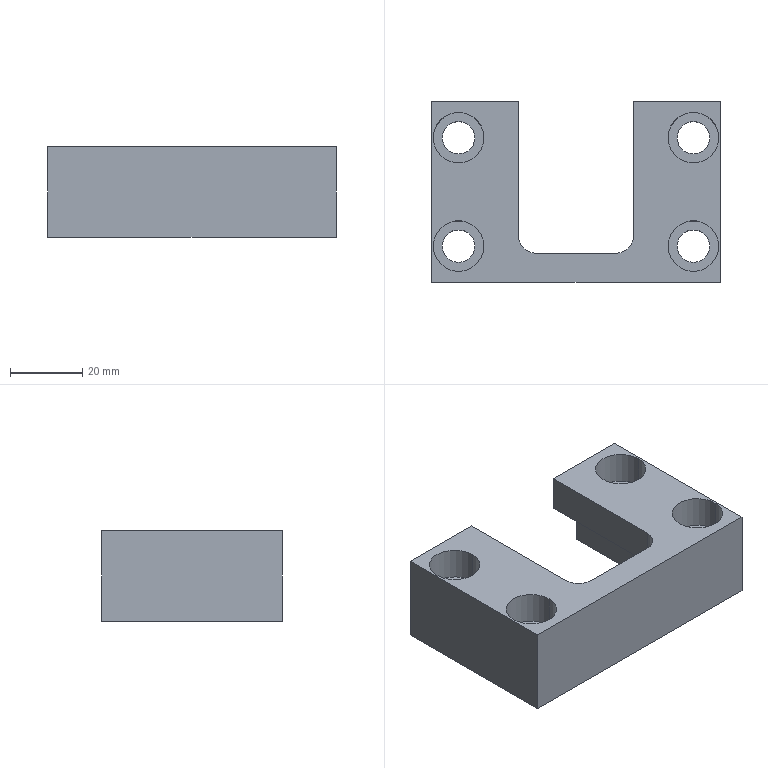Part | SolidWorks | features BaseBody 1 | 1 solid | 38 faces | box 80 x 50 x 25 mm | volume 45715 mm3 | cylinder 20 | plane 18 | commonest cylinder face diameters 9 x8 14 x8 10 x4
STEP:
#1=CARTESIAN_POINT('',(25.5,15.,3.5));
#2=VERTEX_POINT('',#1);
#3=CARTESIAN_POINT('',(39.5,15.,3.5));
#4=VERTEX_POINT('',#3);
#5=CARTESIAN_POINT('',(32.5,15.,3.5));
#6=DIRECTION('',(0.,0.,1.));
#7=DIRECTION('',(1.,0.,0.));
#8=AXIS2_PLACEMENT_3D('',#5,#6,#7);
#9=CIRCLE('',#8,7.);
#10=EDGE_CURVE('',#2,#4,#9,.T.);
#11=ORIENTED_EDGE('',*,*,#10,.F.);
#12=CARTESIAN_POINT('',(25.5,15.,12.5));
#13=VERTEX_POINT('',#12);
#14=CARTESIAN_POINT('',(25.5,15.,12.5));
#15=DIRECTION('',(0.,0.,1.));
#16=VECTOR('',#15,1000.);
#17=LINE('',#14,#16);
#18=EDGE_CURVE('',#2,#13,#17,.T.);
#19=ORIENTED_EDGE('',*,*,#18,.T.);
#20=CARTESIAN_POINT('',(39.5,15.,12.5));
#21=VERTEX_POINT('',#20);
#22=CARTESIAN_POINT('',(32.5,15.,12.5));
#23=DIRECTION('',(0.,0.,1.));
#24=DIRECTION('',(1.,0.,0.));
#25=AXIS2_PLACEMENT_3D('',#22,#23,#24);
#26=CIRCLE('',#25,7.);
#27=EDGE_CURVE('',#13,#21,#26,.T.);
#28=ORIENTED_EDGE('',*,*,#27,.T.);
#29=CARTESIAN_POINT('',(39.5,15.,12.5));
#30=DIRECTION('',(0.,0.,1.));
#31=VECTOR('',#30,1000.);
#32=LINE('',#29,#31);
#33=EDGE_CURVE('',#4,#21,#32,.T.);
#34=ORIENTED_EDGE('',*,*,#33,.F.);
#35=EDGE_LOOP('',(#11,#19,#28,#34));
#36=FACE_OUTER_BOUND('',#35,.T.);
#37=CARTESIAN_POINT('',(32.5,15.,12.5));
#38=DIRECTION('',(0.,0.,1.));
#39=DIRECTION('',(1.,0.,0.));
#40=AXIS2_PLACEMENT_3D('',#37,#38,#39);
#41=CYLINDRICAL_SURFACE('',#40,7.);
#42=ADVANCED_FACE('',(#36),#41,.F.);
#43=CARTESIAN_POINT('',(28.,15.,-12.5));
#44=VERTEX_POINT('',#43);
#45=CARTESIAN_POINT('',(37.,15.,-12.5));
#46=VERTEX_POINT('',#45);
#47=CARTESIAN_POINT('',(32.5,15.,-12.5));
#48=DIRECTION('',(0.,0.,1.));
#49=DIRECTION('',(1.,0.,0.));
#50=AXIS2_PLACEMENT_3D('',#47,#48,#49);
#51=CIRCLE('',#50,4.5);
#52=EDGE_CURVE('',#44,#46,#51,.T.);
#53=ORIENTED_EDGE('',*,*,#52,.F.);
#54=CARTESIAN_POINT('',(28.,15.,3.5));
#55=VERTEX_POINT('',#54);
#56=CARTESIAN_POINT('',(28.,15.,12.5));
#57=DIRECTION('',(0.,0.,1.));
#58=VECTOR('',#57,1000.);
#59=LINE('',#56,#58);
#60=EDGE_CURVE('',#44,#55,#59,.T.);
#61=ORIENTED_EDGE('',*,*,#60,.T.);
#62=CARTESIAN_POINT('',(37.,15.,3.5));
#63=VERTEX_POINT('',#62);
#64=CARTESIAN_POINT('',(32.5,15.,3.5));
#65=DIRECTION('',(0.,0.,1.));
#66=DIRECTION('',(1.,0.,0.));
#67=AXIS2_PLACEMENT_3D('',#64,#65,#66);
#68=CIRCLE('',#67,4.5);
#69=EDGE_CURVE('',#55,#63,#68,.T.);
#70=ORIENTED_EDGE('',*,*,#69,.T.);
#71=CARTESIAN_POINT('',(37.,15.,12.5));
#72=DIRECTION('',(0.,0.,1.));
#73=VECTOR('',#72,1000.);
#74=LINE('',#71,#73);
#75=EDGE_CURVE('',#46,#63,#74,.T.);
#76=ORIENTED_EDGE('',*,*,#75,.F.);
#77=EDGE_LOOP('',(#53,#61,#70,#76));
#78=FACE_OUTER_BOUND('',#77,.T.);
#79=CARTESIAN_POINT('',(32.5,15.,12.5));
#80=DIRECTION('',(0.,0.,1.));
#81=DIRECTION('',(1.,0.,0.));
#82=AXIS2_PLACEMENT_3D('',#79,#80,#81);
#83=CYLINDRICAL_SURFACE('',#82,4.5);
#84=ADVANCED_FACE('',(#78),#83,.F.);
#85=CARTESIAN_POINT('',(25.5,-15.,3.5));
#86=VERTEX_POINT('',#85);
#87=CARTESIAN_POINT('',(39.5,-15.,3.5));
#88=VERTEX_POINT('',#87);
#89=CARTESIAN_POINT('',(32.5,-15.,3.5));
#90=DIRECTION('',(0.,0.,1.));
#91=DIRECTION('',(1.,0.,0.));
#92=AXIS2_PLACEMENT_3D('',#89,#90,#91);
#93=CIRCLE('',#92,7.);
#94=EDGE_CURVE('',#86,#88,#93,.T.);
#95=ORIENTED_EDGE('',*,*,#94,.F.);
#96=CARTESIAN_POINT('',(25.5,-15.,12.5));
#97=VERTEX_POINT('',#96);
#98=CARTESIAN_POINT('',(25.5,-15.,12.5));
#99=DIRECTION('',(0.,0.,1.));
#100=VECTOR('',#99,1000.);
#101=LINE('',#98,#100);
#102=EDGE_CURVE('',#86,#97,#101,.T.);
#103=ORIENTED_EDGE('',*,*,#102,.T.);
#104=CARTESIAN_POINT('',(39.5,-15.,12.5));
#105=VERTEX_POINT('',#104);
#106=CARTESIAN_POINT('',(32.5,-15.,12.5));
#107=DIRECTION('',(0.,0.,1.));
#108=DIRECTION('',(1.,0.,0.));
#109=AXIS2_PLACEMENT_3D('',#106,#107,#108);
#110=CIRCLE('',#109,7.);
#111=EDGE_CURVE('',#97,#105,#110,.T.);
#112=ORIENTED_EDGE('',*,*,#111,.T.);
#113=CARTESIAN_POINT('',(39.5,-15.,12.5));
#114=DIRECTION('',(0.,0.,1.));
#115=VECTOR('',#114,1000.);
#116=LINE('',#113,#115);
#117=EDGE_CURVE('',#88,#105,#116,.T.);
#118=ORIENTED_EDGE('',*,*,#117,.F.);
#119=EDGE_LOOP('',(#95,#103,#112,#118));
#120=FACE_OUTER_BOUND('',#119,.T.);
#121=CARTESIAN_POINT('',(32.5,-15.,12.5));
#122=DIRECTION('',(0.,0.,1.));
#123=DIRECTION('',(1.,0.,0.));
#124=AXIS2_PLACEMENT_3D('',#121,#122,#123);
#125=CYLINDRICAL_SURFACE('',#124,7.);
#126=ADVANCED_FACE('',(#120),#125,.F.);
#127=CARTESIAN_POINT('',(28.,-15.,-12.5));
#128=VERTEX_POINT('',#127);
#129=CARTESIAN_POINT('',(37.,-15.,-12.5));
#130=VERTEX_POINT('',#129);
#131=CARTESIAN_POINT('',(32.5,-15.,-12.5));
#132=DIRECTION('',(0.,0.,1.));
#133=DIRECTION('',(1.,0.,0.));
#134=AXIS2_PLACEMENT_3D('',#131,#132,#133);
#135=CIRCLE('',#134,4.5);
#136=EDGE_CURVE('',#128,#130,#135,.T.);
#137=ORIENTED_EDGE('',*,*,#136,.F.);
#138=CARTESIAN_POINT('',(28.,-15.,3.5));
#139=VERTEX_POINT('',#138);
#140=CARTESIAN_POINT('',(28.,-15.,12.5));
#141=DIRECTION('',(0.,0.,1.));
#142=VECTOR('',#141,1000.);
#143=LINE('',#140,#142);
#144=EDGE_CURVE('',#128,#139,#143,.T.);
#145=ORIENTED_EDGE('',*,*,#144,.T.);
#146=CARTESIAN_POINT('',(37.,-15.,3.5));
#147=VERTEX_POINT('',#146);
#148=CARTESIAN_POINT('',(32.5,-15.,3.5));
#149=DIRECTION('',(0.,0.,1.));
#150=DIRECTION('',(1.,0.,0.));
#151=AXIS2_PLACEMENT_3D('',#148,#149,#150);
#152=CIRCLE('',#151,4.5);
#153=EDGE_CURVE('',#139,#147,#152,.T.);
#154=ORIENTED_EDGE('',*,*,#153,.T.);
#155=CARTESIAN_POINT('',(37.,-15.,12.5));
#156=DIRECTION('',(0.,0.,1.));
#157=VECTOR('',#156,1000.);
#158=LINE('',#155,#157);
#159=EDGE_CURVE('',#130,#147,#158,.T.);
#160=ORIENTED_EDGE('',*,*,#159,.F.);
#161=EDGE_LOOP('',(#137,#145,#154,#160));
#162=FACE_OUTER_BOUND('',#161,.T.);
#163=CARTESIAN_POINT('',(32.5,-15.,12.5));
#164=DIRECTION('',(0.,0.,1.));
#165=DIRECTION('',(1.,0.,0.));
#166=AXIS2_PLACEMENT_3D('',#163,#164,#165);
#167=CYLINDRICAL_SURFACE('',#166,4.5);
#168=ADVANCED_FACE('',(#162),#167,.F.);
#169=CARTESIAN_POINT('',(-39.5,15.,3.5));
#170=VERTEX_POINT('',#169);
#171=CARTESIAN_POINT('',(-25.5,15.,3.5));
#172=VERTEX_POINT('',#171);
#173=CARTESIAN_POINT('',(-32.5,15.,3.5));
#174=DIRECTION('',(0.,0.,1.));
#175=DIRECTION('',(1.,0.,0.));
#176=AXIS2_PLACEMENT_3D('',#173,#174,#175);
#177=CIRCLE('',#176,7.);
#178=EDGE_CURVE('',#170,#172,#177,.T.);
#179=ORIENTED_EDGE('',*,*,#178,.F.);
#180=CARTESIAN_POINT('',(-39.5,15.,12.5));
#181=VERTEX_POINT('',#180);
#182=CARTESIAN_POINT('',(-39.5,15.,12.5));
#183=DIRECTION('',(0.,0.,1.));
#184=VECTOR('',#183,1000.);
#185=LINE('',#182,#184);
#186=EDGE_CURVE('',#170,#181,#185,.T.);
#187=ORIENTED_EDGE('',*,*,#186,.T.);
#188=CARTESIAN_POINT('',(-25.5,15.,12.5));
#189=VERTEX_POINT('',#188);
#190=CARTESIAN_POINT('',(-32.5,15.,12.5));
#191=DIRECTION('',(0.,0.,1.));
#192=DIRECTION('',(1.,0.,0.));
#193=AXIS2_PLACEMENT_3D('',#190,#191,#192);
#194=CIRCLE('',#193,7.);
#195=EDGE_CURVE('',#181,#189,#194,.T.);
#196=ORIENTED_EDGE('',*,*,#195,.T.);
#197=CARTESIAN_POINT('',(-25.5,15.,12.5));
#198=DIRECTION('',(0.,0.,1.));
#199=VECTOR('',#198,1000.);
#200=LINE('',#197,#199);
#201=EDGE_CURVE('',#172,#189,#200,.T.);
#202=ORIENTED_EDGE('',*,*,#201,.F.);
#203=EDGE_LOOP('',(#179,#187,#196,#202));
#204=FACE_OUTER_BOUND('',#203,.T.);
#205=CARTESIAN_POINT('',(-32.5,15.,12.5));
#206=DIRECTION('',(0.,0.,1.));
#207=DIRECTION('',(1.,0.,0.));
#208=AXIS2_PLACEMENT_3D('',#205,#206,#207);
#209=CYLINDRICAL_SURFACE('',#208,7.);
#210=ADVANCED_FACE('',(#204),#209,.F.);
#211=CARTESIAN_POINT('',(-37.,15.,-12.5));
#212=VERTEX_POINT('',#211);
#213=CARTESIAN_POINT('',(-28.,15.,-12.5));
#214=VERTEX_POINT('',#213);
#215=CARTESIAN_POINT('',(-32.5,15.,-12.5));
#216=DIRECTION('',(0.,0.,1.));
#217=DIRECTION('',(1.,0.,0.));
#218=AXIS2_PLACEMENT_3D('',#215,#216,#217);
#219=CIRCLE('',#218,4.5);
#220=EDGE_CURVE('',#212,#214,#219,.T.);
#221=ORIENTED_EDGE('',*,*,#220,.F.);
#222=CARTESIAN_POINT('',(-37.,15.,3.5));
#223=VERTEX_POINT('',#222);
#224=CARTESIAN_POINT('',(-37.,15.,12.5));
#225=DIRECTION('',(0.,0.,1.));
#226=VECTOR('',#225,1000.);
#227=LINE('',#224,#226);
#228=EDGE_CURVE('',#212,#223,#227,.T.);
#229=ORIENTED_EDGE('',*,*,#228,.T.);
#230=CARTESIAN_POINT('',(-28.,15.,3.5));
#231=VERTEX_POINT('',#230);
#232=CARTESIAN_POINT('',(-32.5,15.,3.5));
#233=DIRECTION('',(0.,0.,1.));
#234=DIRECTION('',(1.,0.,0.));
#235=AXIS2_PLACEMENT_3D('',#232,#233,#234);
#236=CIRCLE('',#235,4.5);
#237=EDGE_CURVE('',#223,#231,#236,.T.);
#238=ORIENTED_EDGE('',*,*,#237,.T.);
#239=CARTESIAN_POINT('',(-28.,15.,12.5));
#240=DIRECTION('',(0.,0.,1.));
#241=VECTOR('',#240,1000.);
#242=LINE('',#239,#241);
#243=EDGE_CURVE('',#214,#231,#242,.T.);
#244=ORIENTED_EDGE('',*,*,#243,.F.);
#245=EDGE_LOOP('',(#221,#229,#238,#244));
#246=FACE_OUTER_BOUND('',#245,.T.);
#247=CARTESIAN_POINT('',(-32.5,15.,12.5));
#248=DIRECTION('',(0.,0.,1.));
#249=DIRECTION('',(1.,0.,0.));
#250=AXIS2_PLACEMENT_3D('',#247,#248,#249);
#251=CYLINDRICAL_SURFACE('',#250,4.5);
#252=ADVANCED_FACE('',(#246),#251,.F.);
#253=CARTESIAN_POINT('',(-39.5,-15.,3.5));
#254=VERTEX_POINT('',#253);
#255=CARTESIAN_POINT('',(-25.5,-15.,3.5));
#256=VERTEX_POINT('',#255);
#257=CARTESIAN_POINT('',(-32.5,-15.,3.5));
#258=DIRECTION('',(0.,0.,1.));
#259=DIRECTION('',(1.,0.,0.));
#260=AXIS2_PLACEMENT_3D('',#257,#258,#259);
#261=CIRCLE('',#260,7.);
#262=EDGE_CURVE('',#254,#256,#261,.T.);
#263=ORIENTED_EDGE('',*,*,#262,.F.);
#264=CARTESIAN_POINT('',(-39.5,-15.,12.5));
#265=VERTEX_POINT('',#264);
#266=CARTESIAN_POINT('',(-39.5,-15.,12.5));
#267=DIRECTION('',(0.,0.,1.));
#268=VECTOR('',#267,1000.);
#269=LINE('',#266,#268);
#270=EDGE_CURVE('',#254,#265,#269,.T.);
#271=ORIENTED_EDGE('',*,*,#270,.T.);
#272=CARTESIAN_POINT('',(-25.5,-15.,12.5));
#273=VERTEX_POINT('',#272);
#274=CARTESIAN_POINT('',(-32.5,-15.,12.5));
#275=DIRECTION('',(0.,0.,1.));
#276=DIRECTION('',(1.,0.,0.));
#277=AXIS2_PLACEMENT_3D('',#274,#275,#276);
#278=CIRCLE('',#277,7.);
#279=EDGE_CURVE('',#265,#273,#278,.T.);
#280=ORIENTED_EDGE('',*,*,#279,.T.);
#281=CARTESIAN_POINT('',(-25.5,-15.,12.5));
#282=DIRECTION('',(0.,0.,1.));
#283=VECTOR('',#282,1000.);
#284=LINE('',#281,#283);
#285=EDGE_CURVE('',#256,#273,#284,.T.);
#286=ORIENTED_EDGE('',*,*,#285,.F.);
#287=EDGE_LOOP('',(#263,#271,#280,#286));
#288=FACE_OUTER_BOUND('',#287,.T.);
#289=CARTESIAN_POINT('',(-32.5,-15.,12.5));
#290=DIRECTION('',(0.,0.,1.));
#291=DIRECTION('',(1.,0.,0.));
#292=AXIS2_PLACEMENT_3D('',#289,#290,#291);
#293=CYLINDRICAL_SURFACE('',#292,7.);
#294=ADVANCED_FACE('',(#288),#293,.F.);
#295=CARTESIAN_POINT('',(-37.,-15.,-12.5));
#296=VERTEX_POINT('',#295);
#297=CARTESIAN_POINT('',(-28.,-15.,-12.5));
#298=VERTEX_POINT('',#297);
#299=CARTESIAN_POINT('',(-32.5,-15.,-12.5));
#300=DIRECTION('',(0.,0.,1.));
#301=DIRECTION('',(1.,0.,0.));
#302=AXIS2_PLACEMENT_3D('',#299,#300,#301);
#303=CIRCLE('',#302,4.5);
#304=EDGE_CURVE('',#296,#298,#303,.T.);
#305=ORIENTED_EDGE('',*,*,#304,.F.);
#306=CARTESIAN_POINT('',(-37.,-15.,3.5));
#307=VERTEX_POINT('',#306);
#308=CARTESIAN_POINT('',(-37.,-15.,12.5));
#309=DIRECTION('',(0.,0.,1.));
#310=VECTOR('',#309,1000.);
#311=LINE('',#308,#310);
#312=EDGE_CURVE('',#296,#307,#311,.T.);
#313=ORIENTED_EDGE('',*,*,#312,.T.);
#314=CARTESIAN_POINT('',(-28.,-15.,3.5));
#315=VERTEX_POINT('',#314);
#316=CARTESIAN_POINT('',(-32.5,-15.,3.5));
#317=DIRECTION('',(0.,0.,1.));
#318=DIRECTION('',(1.,0.,0.));
#319=AXIS2_PLACEMENT_3D('',#316,#317,#318);
#320=CIRCLE('',#319,4.5);
#321=EDGE_CURVE('',#307,#315,#320,.T.);
#322=ORIENTED_EDGE('',*,*,#321,.T.);
#323=CARTESIAN_POINT('',(-28.,-15.,12.5));
#324=DIRECTION('',(0.,0.,1.));
#325=VECTOR('',#324,1000.);
#326=LINE('',#323,#325);
#327=EDGE_CURVE('',#298,#315,#326,.T.);
#328=ORIENTED_EDGE('',*,*,#327,.F.);
#329=EDGE_LOOP('',(#305,#313,#322,#328));
#330=FACE_OUTER_BOUND('',#329,.T.);
#331=CARTESIAN_POINT('',(-32.5,-15.,12.5));
#332=DIRECTION('',(0.,0.,1.));
#333=DIRECTION('',(1.,0.,0.));
#334=AXIS2_PLACEMENT_3D('',#331,#332,#333);
#335=CYLINDRICAL_SURFACE('',#334,4.5);
#336=ADVANCED_FACE('',(#330),#335,.F.);
#337=CARTESIAN_POINT('',(16.,25.,2.5));
#338=VERTEX_POINT('',#337);
#339=CARTESIAN_POINT('',(25.,25.,2.5));
#340=VERTEX_POINT('',#339);
#341=CARTESIAN_POINT('',(25.,25.,2.5));
#342=DIRECTION('',(1.,0.,0.));
#343=VECTOR('',#342,1000.);
#344=LINE('',#341,#343);
#345=EDGE_CURVE('',#338,#340,#344,.T.);
#346=ORIENTED_EDGE('',*,*,#345,.F.);
#347=CARTESIAN_POINT('',(16.,25.,12.5));
#348=VERTEX_POINT('',#347);
#349=CARTESIAN_POINT('',(16.,25.,12.5));
#350=DIRECTION('',(0.,0.,-1.));
#351=VECTOR('',#350,1000.);
#352=LINE('',#349,#351);
#353=EDGE_CURVE('',#348,#338,#352,.T.);
#354=ORIENTED_EDGE('',*,*,#353,.F.);
#355=CARTESIAN_POINT('',(40.,25.,12.5));
#356=VERTEX_POINT('',#355);
#357=CARTESIAN_POINT('',(40.,25.,12.5));
#358=DIRECTION('',(-1.,0.,0.));
#359=VECTOR('',#358,1000.);
#360=LINE('',#357,#359);
#361=EDGE_CURVE('',#356,#348,#360,.T.);
#362=ORIENTED_EDGE('',*,*,#361,.F.);
#363=CARTESIAN_POINT('',(40.,25.,-12.5));
#364=VERTEX_POINT('',#363);
#365=CARTESIAN_POINT('',(40.,25.,12.5));
#366=DIRECTION('',(0.,0.,-1.));
#367=VECTOR('',#366,1000.);
#368=LINE('',#365,#367);
#369=EDGE_CURVE('',#356,#364,#368,.T.);
#370=ORIENTED_EDGE('',*,*,#369,.T.);
#371=CARTESIAN_POINT('',(25.,25.,-12.5));
#372=VERTEX_POINT('',#371);
#373=CARTESIAN_POINT('',(40.,25.,-12.5));
#374=DIRECTION('',(-1.,0.,0.));
#375=VECTOR('',#374,1000.);
#376=LINE('',#373,#375);
#377=EDGE_CURVE('',#364,#372,#376,.T.);
#378=ORIENTED_EDGE('',*,*,#377,.T.);
#379=CARTESIAN_POINT('',(25.,25.,2.5));
#380=DIRECTION('',(0.,0.,-1.));
#381=VECTOR('',#380,1000.);
#382=LINE('',#379,#381);
#383=EDGE_CURVE('',#340,#372,#382,.T.);
#384=ORIENTED_EDGE('',*,*,#383,.F.);
#385=EDGE_LOOP('',(#346,#354,#362,#370,#378,#384));
#386=FACE_OUTER_BOUND('',#385,.T.);
#387=CARTESIAN_POINT('',(40.,25.,12.5));
#388=DIRECTION('',(0.,-1.,0.));
#389=DIRECTION('',(1.,0.,0.));
#390=AXIS2_PLACEMENT_3D('',#387,#388,#389);
#391=PLANE('',#390);
#392=ADVANCED_FACE('',(#386),#391,.F.);
#393=CARTESIAN_POINT('',(16.,-12.,2.5));
#394=VERTEX_POINT('',#393);
#395=CARTESIAN_POINT('',(16.,25.,2.5));
#396=DIRECTION('',(0.,-1.,0.));
#397=VECTOR('',#396,1000.);
#398=LINE('',#395,#397);
#399=EDGE_CURVE('',#338,#394,#398,.T.);
#400=ORIENTED_EDGE('',*,*,#399,.F.);
#401=ORIENTED_EDGE('',*,*,#345,.T.);
#402=CARTESIAN_POINT('',(25.,-12.,2.5));
#403=VERTEX_POINT('',#402);
#404=CARTESIAN_POINT('',(25.,25.,2.5));
#405=DIRECTION('',(0.,-1.,0.));
#406=VECTOR('',#405,1000.);
#407=LINE('',#404,#406);
#408=EDGE_CURVE('',#340,#403,#407,.T.);
#409=ORIENTED_EDGE('',*,*,#408,.T.);
#410=CARTESIAN_POINT('',(20.,-17.,2.5));
#411=VERTEX_POINT('',#410);
#412=CARTESIAN_POINT('',(20.,-12.,2.5));
#413=DIRECTION('',(0.,0.,-1.));
#414=DIRECTION('',(-1.,0.,0.));
#415=AXIS2_PLACEMENT_3D('',#412,#413,#414);
#416=CIRCLE('',#415,5.);
#417=EDGE_CURVE('',#403,#411,#416,.T.);
#418=ORIENTED_EDGE('',*,*,#417,.T.);
#419=CARTESIAN_POINT('',(11.,-17.,2.5));
#420=VERTEX_POINT('',#419);
#421=CARTESIAN_POINT('',(20.,-17.,2.5));
#422=DIRECTION('',(-1.,0.,0.));
#423=VECTOR('',#422,1000.);
#424=LINE('',#421,#423);
#425=EDGE_CURVE('',#411,#420,#424,.T.);
#426=ORIENTED_EDGE('',*,*,#425,.T.);
#427=CARTESIAN_POINT('',(11.,-12.,2.5));
#428=DIRECTION('',(0.,0.,1.));
#429=DIRECTION('',(-1.,0.,0.));
#430=AXIS2_PLACEMENT_3D('',#427,#428,#429);
#431=CIRCLE('',#430,5.);
#432=EDGE_CURVE('',#420,#394,#431,.T.);
#433=ORIENTED_EDGE('',*,*,#432,.T.);
#434=EDGE_LOOP('',(#400,#401,#409,#418,#426,#433));
#435=FACE_OUTER_BOUND('',#434,.T.);
#436=CARTESIAN_POINT('',(20.,-12.,2.5));
#437=DIRECTION('',(0.,0.,-1.));
#438=DIRECTION('',(-1.,0.,0.));
#439=AXIS2_PLACEMENT_3D('',#436,#437,#438);
#440=PLANE('',#439);
#441=ADVANCED_FACE('',(#435),#440,.T.);
#442=CARTESIAN_POINT('',(-40.,25.,-12.5));
#443=VERTEX_POINT('',#442);
#444=CARTESIAN_POINT('',(-40.,-25.,-12.5));
#445=VERTEX_POINT('',#444);
#446=CARTESIAN_POINT('',(-40.,25.,-12.5));
#447=DIRECTION('',(0.,-1.,0.));
#448=VECTOR('',#447,1000.);
#449=LINE('',#446,#448);
#450=EDGE_CURVE('',#443,#445,#449,.T.);
#451=ORIENTED_EDGE('',*,*,#450,.T.);
#452=CARTESIAN_POINT('',(-40.,-25.,12.5));
#453=VERTEX_POINT('',#452);
#454=CARTESIAN_POINT('',(-40.,-25.,12.5));
#455=DIRECTION('',(0.,0.,-1.));
#456=VECTOR('',#455,1000.);
#457=LINE('',#454,#456);
#458=EDGE_CURVE('',#453,#445,#457,.T.);
#459=ORIENTED_EDGE('',*,*,#458,.F.);
#460=CARTESIAN_POINT('',(-40.,25.,12.5));
#461=VERTEX_POINT('',#460);
#462=CARTESIAN_POINT('',(-40.,25.,12.5));
#463=DIRECTION('',(0.,-1.,0.));
#464=VECTOR('',#463,1000.);
#465=LINE('',#462,#464);
#466=EDGE_CURVE('',#461,#453,#465,.T.);
#467=ORIENTED_EDGE('',*,*,#466,.F.);
#468=CARTESIAN_POINT('',(-40.,25.,12.5));
#469=DIRECTION('',(0.,0.,-1.));
#470=VECTOR('',#469,1000.);
#471=LINE('',#468,#470);
#472=EDGE_CURVE('',#461,#443,#471,.T.);
#473=ORIENTED_EDGE('',*,*,#472,.T.);
#474=EDGE_LOOP('',(#451,#459,#467,#473));
#475=FACE_OUTER_BOUND('',#474,.T.);
#476=CARTESIAN_POINT('',(-40.,25.,12.5));
#477=DIRECTION('',(1.,0.,0.));
#478=DIRECTION('',(0.,1.,0.));
#479=AXIS2_PLACEMENT_3D('',#476,#477,#478);
#480=PLANE('',#479);
#481=ADVANCED_FACE('',(#475),#480,.F.);
#482=CARTESIAN_POINT('',(40.,-25.,-12.5));
#483=VERTEX_POINT('',#482);
#484=CARTESIAN_POINT('',(40.,-25.,-12.5));
#485=DIRECTION('',(1.,0.,0.));
#486=VECTOR('',#485,1000.);
#487=LINE('',#484,#486);
#488=EDGE_CURVE('',#445,#483,#487,.T.);
#489=ORIENTED_EDGE('',*,*,#488,.T.);
#490=CARTESIAN_POINT('',(40.,-25.,12.5));
#491=VERTEX_POINT('',#490);
#492=CARTESIAN_POINT('',(40.,-25.,12.5));
#493=DIRECTION('',(0.,0.,-1.));
#494=VECTOR('',#493,1000.);
#495=LINE('',#492,#494);
#496=EDGE_CURVE('',#491,#483,#495,.T.);
#497=ORIENTED_EDGE('',*,*,#496,.F.);
#498=CARTESIAN_POINT('',(40.,-25.,12.5));
#499=DIRECTION('',(1.,0.,0.));
#500=VECTOR('',#499,1000.);
#501=LINE('',#498,#500);
#502=EDGE_CURVE('',#453,#491,#501,.T.);
#503=ORIENTED_EDGE('',*,*,#502,.F.);
#504=ORIENTED_EDGE('',*,*,#458,.T.);
#505=EDGE_LOOP('',(#489,#497,#503,#504));
#506=FACE_OUTER_BOUND('',#505,.T.);
#507=CARTESIAN_POINT('',(40.,-25.,12.5));
#508=DIRECTION('',(0.,1.,0.));
#509=DIRECTION('',(-1.,0.,0.));
#510=AXIS2_PLACEMENT_3D('',#507,#508,#509);
#511=PLANE('',#510);
#512=ADVANCED_FACE('',(#506),#511,.F.);
#513=CARTESIAN_POINT('',(40.,25.,-12.5));
#514=DIRECTION('',(0.,1.,0.));
#515=VECTOR('',#514,1000.);
#516=LINE('',#513,#515);
#517=EDGE_CURVE('',#483,#364,#516,.T.);
#518=ORIENTED_EDGE('',*,*,#517,.T.);
#519=ORIENTED_EDGE('',*,*,#369,.F.);
#520=CARTESIAN_POINT('',(40.,25.,12.5));
#521=DIRECTION('',(0.,1.,0.));
#522=VECTOR('',#521,1000.);
#523=LINE('',#520,#522);
#524=EDGE_CURVE('',#491,#356,#523,.T.);
#525=ORIENTED_EDGE('',*,*,#524,.F.);
#526=ORIENTED_EDGE('',*,*,#496,.T.);
#527=EDGE_LOOP('',(#518,#519,#525,#526));
#528=FACE_OUTER_BOUND('',#527,.T.);
#529=CARTESIAN_POINT('',(40.,25.,12.5));
#530=DIRECTION('',(-1.,0.,0.));
#531=DIRECTION('',(0.,0.,1.));
#532=AXIS2_PLACEMENT_3D('',#529,#530,#531);
#533=PLANE('',#532);
#534=ADVANCED_FACE('',(#528),#533,.F.);
#535=CARTESIAN_POINT('',(-16.,25.,12.5));
#536=VERTEX_POINT('',#535);
#537=CARTESIAN_POINT('',(40.,25.,12.5));
#538=DIRECTION('',(-1.,0.,0.));
#539=VECTOR('',#538,1000.);
#540=LINE('',#537,#539);
#541=EDGE_CURVE('',#536,#461,#540,.T.);
#542=ORIENTED_EDGE('',*,*,#541,.F.);
#543=CARTESIAN_POINT('',(-16.,25.,2.5));
#544=VERTEX_POINT('',#543);
#545=CARTESIAN_POINT('',(-16.,25.,12.5));
#546=DIRECTION('',(0.,0.,-1.));
#547=VECTOR('',#546,1000.);
#548=LINE('',#545,#547);
#549=EDGE_CURVE('',#536,#544,#548,.T.);
#550=ORIENTED_EDGE('',*,*,#549,.T.);
#551=CARTESIAN_POINT('',(-25.,25.,2.5));
#552=VERTEX_POINT('',#551);
#553=CARTESIAN_POINT('',(25.,25.,2.5));
#554=DIRECTION('',(1.,0.,0.));
#555=VECTOR('',#554,1000.);
#556=LINE('',#553,#555);
#557=EDGE_CURVE('',#552,#544,#556,.T.);
#558=ORIENTED_EDGE('',*,*,#557,.F.);
#559=CARTESIAN_POINT('',(-25.,25.,-12.5));
#560=VERTEX_POINT('',#559);
#561=CARTESIAN_POINT('',(-25.,25.,2.5));
#562=DIRECTION('',(0.,0.,-1.));
#563=VECTOR('',#562,1000.);
#564=LINE('',#561,#563);
#565=EDGE_CURVE('',#552,#560,#564,.T.);
#566=ORIENTED_EDGE('',*,*,#565,.T.);
#567=CARTESIAN_POINT('',(40.,25.,-12.5));
#568=DIRECTION('',(-1.,0.,0.));
#569=VECTOR('',#568,1000.);
#570=LINE('',#567,#569);
#571=EDGE_CURVE('',#560,#443,#570,.T.);
#572=ORIENTED_EDGE('',*,*,#571,.T.);
#573=ORIENTED_EDGE('',*,*,#472,.F.);
#574=EDGE_LOOP('',(#542,#550,#558,#566,#572,#573));
#575=FACE_OUTER_BOUND('',#574,.T.);
#576=CARTESIAN_POINT('',(40.,25.,12.5));
#577=DIRECTION('',(0.,-1.,0.));
#578=DIRECTION('',(1.,0.,0.));
#579=AXIS2_PLACEMENT_3D('',#576,#577,#578);
#580=PLANE('',#579);
#581=ADVANCED_FACE('',(#575),#580,.F.);
#582=CARTESIAN_POINT('',(32.5,15.,12.5));
#583=DIRECTION('',(0.,0.,1.));
#584=DIRECTION('',(1.,0.,0.));
#585=AXIS2_PLACEMENT_3D('',#582,#583,#584);
#586=CIRCLE('',#585,7.);
#587=EDGE_CURVE('',#21,#13,#586,.T.);
#588=ORIENTED_EDGE('',*,*,#587,.F.);
#589=ORIENTED_EDGE('',*,*,#27,.F.);
#590=EDGE_LOOP('',(#588,#589));
#591=FACE_BOUND('',#590,.T.);
#592=CARTESIAN_POINT('',(32.5,-15.,12.5));
#593=DIRECTION('',(0.,0.,1.));
#594=DIRECTION('',(1.,0.,0.));
#595=AXIS2_PLACEMENT_3D('',#592,#593,#594);
#596=CIRCLE('',#595,7.);
#597=EDGE_CURVE('',#105,#97,#596,.T.);
#598=ORIENTED_EDGE('',*,*,#597,.F.);
#599=ORIENTED_EDGE('',*,*,#111,.F.);
#600=EDGE_LOOP('',(#598,#599));
#601=FACE_BOUND('',#600,.T.);
#602=CARTESIAN_POINT('',(-32.5,15.,12.5));
#603=DIRECTION('',(0.,0.,1.));
#604=DIRECTION('',(1.,0.,0.));
#605=AXIS2_PLACEMENT_3D('',#602,#603,#604);
#606=CIRCLE('',#605,7.);
#607=EDGE_CURVE('',#189,#181,#606,.T.);
#608=ORIENTED_EDGE('',*,*,#607,.F.);
#609=ORIENTED_EDGE('',*,*,#195,.F.);
#610=EDGE_LOOP('',(#608,#609));
#611=FACE_BOUND('',#610,.T.);
#612=CARTESIAN_POINT('',(-32.5,-15.,12.5));
#613=DIRECTION('',(0.,0.,1.));
#614=DIRECTION('',(1.,0.,0.));
#615=AXIS2_PLACEMENT_3D('',#612,#613,#614);
#616=CIRCLE('',#615,7.);
#617=EDGE_CURVE('',#273,#265,#616,.T.);
#618=ORIENTED_EDGE('',*,*,#617,.F.);
#619=ORIENTED_EDGE('',*,*,#279,.F.);
#620=EDGE_LOOP('',(#618,#619));
#621=FACE_BOUND('',#620,.T.);
#622=ORIENTED_EDGE('',*,*,#361,.T.);
#623=CARTESIAN_POINT('',(16.,-12.,12.5));
#624=VERTEX_POINT('',#623);
#625=CARTESIAN_POINT('',(16.,25.,12.5));
#626=DIRECTION('',(0.,-1.,0.));
#627=VECTOR('',#626,1000.);
#628=LINE('',#625,#627);
#629=EDGE_CURVE('',#348,#624,#628,.T.);
#630=ORIENTED_EDGE('',*,*,#629,.T.);
#631=CARTESIAN_POINT('',(11.,-17.,12.5));
#632=VERTEX_POINT('',#631);
#633=CARTESIAN_POINT('',(11.,-12.,12.5));
#634=DIRECTION('',(0.,0.,-1.));
#635=DIRECTION('',(-1.,0.,0.));
#636=AXIS2_PLACEMENT_3D('',#633,#634,#635);
#637=CIRCLE('',#636,5.);
#638=EDGE_CURVE('',#624,#632,#637,.T.);
#639=ORIENTED_EDGE('',*,*,#638,.T.);
#640=CARTESIAN_POINT('',(-11.,-17.,12.5));
#641=VERTEX_POINT('',#640);
#642=CARTESIAN_POINT('',(16.,-17.,12.5));
#643=DIRECTION('',(-1.,0.,0.));
#644=VECTOR('',#643,1000.);
#645=LINE('',#642,#644);
#646=EDGE_CURVE('',#632,#641,#645,.T.);
#647=ORIENTED_EDGE('',*,*,#646,.T.);
#648=CARTESIAN_POINT('',(-16.,-12.,12.5));
#649=VERTEX_POINT('',#648);
#650=CARTESIAN_POINT('',(-11.,-12.,12.5));
#651=DIRECTION('',(0.,0.,-1.));
#652=DIRECTION('',(-1.,0.,0.));
#653=AXIS2_PLACEMENT_3D('',#650,#651,#652);
#654=CIRCLE('',#653,5.);
#655=EDGE_CURVE('',#641,#649,#654,.T.);
#656=ORIENTED_EDGE('',*,*,#655,.T.);
#657=CARTESIAN_POINT('',(-16.,25.,12.5));
#658=DIRECTION('',(0.,1.,0.));
#659=VECTOR('',#658,1000.);
#660=LINE('',#657,#659);
#661=EDGE_CURVE('',#649,#536,#660,.T.);
#662=ORIENTED_EDGE('',*,*,#661,.T.);
#663=ORIENTED_EDGE('',*,*,#541,.T.);
#664=ORIENTED_EDGE('',*,*,#466,.T.);
#665=ORIENTED_EDGE('',*,*,#502,.T.);
#666=ORIENTED_EDGE('',*,*,#524,.T.);
#667=EDGE_LOOP('',(#622,#630,#639,#647,#656,#662,#663,#664,#665,#666));
#668=FACE_OUTER_BOUND('',#667,.T.);
#669=CARTESIAN_POINT('',(-40.,-25.,12.5));
#670=DIRECTION('',(0.,0.,-1.));
#671=DIRECTION('',(-1.,0.,0.));
#672=AXIS2_PLACEMENT_3D('',#669,#670,#671);
#673=PLANE('',#672);
#674=ADVANCED_FACE('',(#591,#601,#611,#621,#668),#673,.F.);
#675=CARTESIAN_POINT('',(32.5,15.,-12.5));
#676=DIRECTION('',(0.,0.,1.));
#677=DIRECTION('',(1.,0.,0.));
#678=AXIS2_PLACEMENT_3D('',#675,#676,#677);
#679=CIRCLE('',#678,4.5);
#680=EDGE_CURVE('',#46,#44,#679,.T.);
#681=ORIENTED_EDGE('',*,*,#680,.T.);
#682=ORIENTED_EDGE('',*,*,#52,.T.);
#683=EDGE_LOOP('',(#681,#682));
#684=FACE_BOUND('',#683,.T.);
#685=CARTESIAN_POINT('',(32.5,-15.,-12.5));
#686=DIRECTION('',(0.,0.,1.));
#687=DIRECTION('',(1.,0.,0.));
#688=AXIS2_PLACEMENT_3D('',#685,#686,#687);
#689=CIRCLE('',#688,4.5);
#690=EDGE_CURVE('',#130,#128,#689,.T.);
#691=ORIENTED_EDGE('',*,*,#690,.T.);
#692=ORIENTED_EDGE('',*,*,#136,.T.);
#693=EDGE_LOOP('',(#691,#692));
#694=FACE_BOUND('',#693,.T.);
#695=CARTESIAN_POINT('',(-32.5,15.,-12.5));
#696=DIRECTION('',(0.,0.,1.));
#697=DIRECTION('',(1.,0.,0.));
#698=AXIS2_PLACEMENT_3D('',#695,#696,#697);
#699=CIRCLE('',#698,4.5);
#700=EDGE_CURVE('',#214,#212,#699,.T.);
#701=ORIENTED_EDGE('',*,*,#700,.T.);
#702=ORIENTED_EDGE('',*,*,#220,.T.);
#703=EDGE_LOOP('',(#701,#702));
#704=FACE_BOUND('',#703,.T.);
#705=CARTESIAN_POINT('',(-32.5,-15.,-12.5));
#706=DIRECTION('',(0.,0.,1.));
#707=DIRECTION('',(1.,0.,0.));
#708=AXIS2_PLACEMENT_3D('',#705,#706,#707);
#709=CIRCLE('',#708,4.5);
#710=EDGE_CURVE('',#298,#296,#709,.T.);
#711=ORIENTED_EDGE('',*,*,#710,.T.);
#712=ORIENTED_EDGE('',*,*,#304,.T.);
#713=EDGE_LOOP('',(#711,#712));
#714=FACE_BOUND('',#713,.T.);
#715=CARTESIAN_POINT('',(25.,-12.,-12.5));
#716=VERTEX_POINT('',#715);
#717=CARTESIAN_POINT('',(25.,25.,-12.5));
#718=DIRECTION('',(0.,-1.,0.));
#719=VECTOR('',#718,1000.);
#720=LINE('',#717,#719);
#721=EDGE_CURVE('',#372,#716,#720,.T.);
#722=ORIENTED_EDGE('',*,*,#721,.F.);
#723=ORIENTED_EDGE('',*,*,#377,.F.);
#724=ORIENTED_EDGE('',*,*,#517,.F.);
#725=ORIENTED_EDGE('',*,*,#488,.F.);
#726=ORIENTED_EDGE('',*,*,#450,.F.);
#727=ORIENTED_EDGE('',*,*,#571,.F.);
#728=CARTESIAN_POINT('',(-25.,-12.,-12.5));
#729=VERTEX_POINT('',#728);
#730=CARTESIAN_POINT('',(-25.,25.,-12.5));
#731=DIRECTION('',(0.,1.,0.));
#732=VECTOR('',#731,1000.);
#733=LINE('',#730,#732);
#734=EDGE_CURVE('',#729,#560,#733,.T.);
#735=ORIENTED_EDGE('',*,*,#734,.F.);
#736=CARTESIAN_POINT('',(-20.,-17.,-12.5));
#737=VERTEX_POINT('',#736);
#738=CARTESIAN_POINT('',(-20.,-12.,-12.5));
#739=DIRECTION('',(0.,0.,-1.));
#740=DIRECTION('',(1.,0.,0.));
#741=AXIS2_PLACEMENT_3D('',#738,#739,#740);
#742=CIRCLE('',#741,5.);
#743=EDGE_CURVE('',#737,#729,#742,.T.);
#744=ORIENTED_EDGE('',*,*,#743,.F.);
#745=CARTESIAN_POINT('',(20.,-17.,-12.5));
#746=VERTEX_POINT('',#745);
#747=CARTESIAN_POINT('',(20.,-17.,-12.5));
#748=DIRECTION('',(-1.,0.,0.));
#749=VECTOR('',#748,1000.);
#750=LINE('',#747,#749);
#751=EDGE_CURVE('',#746,#737,#750,.T.);
#752=ORIENTED_EDGE('',*,*,#751,.F.);
#753=CARTESIAN_POINT('',(20.,-12.,-12.5));
#754=DIRECTION('',(0.,0.,-1.));
#755=DIRECTION('',(-1.,0.,0.));
#756=AXIS2_PLACEMENT_3D('',#753,#754,#755);
#757=CIRCLE('',#756,5.);
#758=EDGE_CURVE('',#716,#746,#757,.T.);
#759=ORIENTED_EDGE('',*,*,#758,.F.);
#760=EDGE_LOOP('',(#722,#723,#724,#725,#726,#727,#735,#744,#752,#759));
#761=FACE_OUTER_BOUND('',#760,.T.);
#762=CARTESIAN_POINT('',(-40.,-25.,-12.5));
#763=DIRECTION('',(0.,0.,-1.));
#764=DIRECTION('',(-1.,0.,0.));
#765=AXIS2_PLACEMENT_3D('',#762,#763,#764);
#766=PLANE('',#765);
#767=ADVANCED_FACE('',(#684,#694,#704,#714,#761),#766,.T.);
#768=ORIENTED_EDGE('',*,*,#721,.T.);
#769=CARTESIAN_POINT('',(25.,-12.,2.5));
#770=DIRECTION('',(0.,0.,-1.));
#771=VECTOR('',#770,1000.);
#772=LINE('',#769,#771);
#773=EDGE_CURVE('',#403,#716,#772,.T.);
#774=ORIENTED_EDGE('',*,*,#773,.F.);
#775=ORIENTED_EDGE('',*,*,#408,.F.);
#776=ORIENTED_EDGE('',*,*,#383,.T.);
#777=EDGE_LOOP('',(#768,#774,#775,#776));
#778=FACE_OUTER_BOUND('',#777,.T.);
#779=CARTESIAN_POINT('',(25.,25.,2.5));
#780=DIRECTION('',(1.,0.,0.));
#781=DIRECTION('',(0.,1.,0.));
#782=AXIS2_PLACEMENT_3D('',#779,#780,#781);
#783=PLANE('',#782);
#784=ADVANCED_FACE('',(#778),#783,.F.);
#785=ORIENTED_EDGE('',*,*,#734,.T.);
#786=ORIENTED_EDGE('',*,*,#565,.F.);
#787=CARTESIAN_POINT('',(-25.,-12.,2.5));
#788=VERTEX_POINT('',#787);
#789=CARTESIAN_POINT('',(-25.,25.,2.5));
#790=DIRECTION('',(0.,1.,0.));
#791=VECTOR('',#790,1000.);
#792=LINE('',#789,#791);
#793=EDGE_CURVE('',#788,#552,#792,.T.);
#794=ORIENTED_EDGE('',*,*,#793,.F.);
#795=CARTESIAN_POINT('',(-25.,-12.,2.5));
#796=DIRECTION('',(0.,0.,-1.));
#797=VECTOR('',#796,1000.);
#798=LINE('',#795,#797);
#799=EDGE_CURVE('',#788,#729,#798,.T.);
#800=ORIENTED_EDGE('',*,*,#799,.T.);
#801=EDGE_LOOP('',(#785,#786,#794,#800));
#802=FACE_OUTER_BOUND('',#801,.T.);
#803=CARTESIAN_POINT('',(-25.,25.,2.5));
#804=DIRECTION('',(-1.,0.,0.));
#805=DIRECTION('',(0.,0.,1.));
#806=AXIS2_PLACEMENT_3D('',#803,#804,#805);
#807=PLANE('',#806);
#808=ADVANCED_FACE('',(#802),#807,.F.);
#809=ORIENTED_EDGE('',*,*,#743,.T.);
#810=ORIENTED_EDGE('',*,*,#799,.F.);
#811=CARTESIAN_POINT('',(-20.,-17.,2.5));
#812=VERTEX_POINT('',#811);
#813=CARTESIAN_POINT('',(-20.,-12.,2.5));
#814=DIRECTION('',(0.,0.,-1.));
#815=DIRECTION('',(1.,0.,0.));
#816=AXIS2_PLACEMENT_3D('',#813,#814,#815);
#817=CIRCLE('',#816,5.);
#818=EDGE_CURVE('',#812,#788,#817,.T.);
#819=ORIENTED_EDGE('',*,*,#818,.F.);
#820=CARTESIAN_POINT('',(-20.,-17.,2.5));
#821=DIRECTION('',(0.,0.,-1.));
#822=VECTOR('',#821,1000.);
#823=LINE('',#820,#822);
#824=EDGE_CURVE('',#812,#737,#823,.T.);
#825=ORIENTED_EDGE('',*,*,#824,.T.);
#826=EDGE_LOOP('',(#809,#810,#819,#825));
#827=FACE_OUTER_BOUND('',#826,.T.);
#828=CARTESIAN_POINT('',(-20.,-12.,2.5));
#829=DIRECTION('',(0.,0.,-1.));
#830=DIRECTION('',(-1.,0.,0.));
#831=AXIS2_PLACEMENT_3D('',#828,#829,#830);
#832=CYLINDRICAL_SURFACE('',#831,5.);
#833=ADVANCED_FACE('',(#827),#832,.F.);
#834=CARTESIAN_POINT('',(-11.,-17.,2.5));
#835=VERTEX_POINT('',#834);
#836=CARTESIAN_POINT('',(20.,-17.,2.5));
#837=DIRECTION('',(-1.,0.,0.));
#838=VECTOR('',#837,1000.);
#839=LINE('',#836,#838);
#840=EDGE_CURVE('',#835,#812,#839,.T.);
#841=ORIENTED_EDGE('',*,*,#840,.F.);
#842=CARTESIAN_POINT('',(-11.,-17.,12.5));
#843=DIRECTION('',(0.,0.,1.));
#844=VECTOR('',#843,1000.);
#845=LINE('',#842,#844);
#846=EDGE_CURVE('',#835,#641,#845,.T.);
#847=ORIENTED_EDGE('',*,*,#846,.T.);
#848=ORIENTED_EDGE('',*,*,#646,.F.);
#849=CARTESIAN_POINT('',(11.,-17.,2.5));
#850=DIRECTION('',(0.,0.,-1.));
#851=VECTOR('',#850,1000.);
#852=LINE('',#849,#851);
#853=EDGE_CURVE('',#632,#420,#852,.T.);
#854=ORIENTED_EDGE('',*,*,#853,.T.);
#855=ORIENTED_EDGE('',*,*,#425,.F.);
#856=CARTESIAN_POINT('',(20.,-17.,2.5));
#857=DIRECTION('',(0.,0.,-1.));
#858=VECTOR('',#857,1000.);
#859=LINE('',#856,#858);
#860=EDGE_CURVE('',#411,#746,#859,.T.);
#861=ORIENTED_EDGE('',*,*,#860,.T.);
#862=ORIENTED_EDGE('',*,*,#751,.T.);
#863=ORIENTED_EDGE('',*,*,#824,.F.);
#864=EDGE_LOOP('',(#841,#847,#848,#854,#855,#861,#862,#863));
#865=FACE_OUTER_BOUND('',#864,.T.);
#866=CARTESIAN_POINT('',(20.,-17.,2.5));
#867=DIRECTION('',(0.,-1.,0.));
#868=DIRECTION('',(1.,0.,0.));
#869=AXIS2_PLACEMENT_3D('',#866,#867,#868);
#870=PLANE('',#869);
#871=ADVANCED_FACE('',(#865),#870,.F.);
#872=ORIENTED_EDGE('',*,*,#758,.T.);
#873=ORIENTED_EDGE('',*,*,#860,.F.);
#874=ORIENTED_EDGE('',*,*,#417,.F.);
#875=ORIENTED_EDGE('',*,*,#773,.T.);
#876=EDGE_LOOP('',(#872,#873,#874,#875));
#877=FACE_OUTER_BOUND('',#876,.T.);
#878=CARTESIAN_POINT('',(20.,-12.,2.5));
#879=DIRECTION('',(0.,0.,-1.));
#880=DIRECTION('',(-1.,0.,0.));
#881=AXIS2_PLACEMENT_3D('',#878,#879,#880);
#882=CYLINDRICAL_SURFACE('',#881,5.);
#883=ADVANCED_FACE('',(#877),#882,.F.);
#884=CARTESIAN_POINT('',(-16.,-12.,2.5));
#885=VERTEX_POINT('',#884);
#886=CARTESIAN_POINT('',(-16.,25.,2.5));
#887=DIRECTION('',(0.,1.,0.));
#888=VECTOR('',#887,1000.);
#889=LINE('',#886,#888);
#890=EDGE_CURVE('',#885,#544,#889,.T.);
#891=ORIENTED_EDGE('',*,*,#890,.F.);
#892=CARTESIAN_POINT('',(-11.,-12.,2.5));
#893=DIRECTION('',(0.,0.,1.));
#894=DIRECTION('',(-1.,0.,0.));
#895=AXIS2_PLACEMENT_3D('',#892,#893,#894);
#896=CIRCLE('',#895,5.);
#897=EDGE_CURVE('',#885,#835,#896,.T.);
#898=ORIENTED_EDGE('',*,*,#897,.T.);
#899=ORIENTED_EDGE('',*,*,#840,.T.);
#900=ORIENTED_EDGE('',*,*,#818,.T.);
#901=ORIENTED_EDGE('',*,*,#793,.T.);
#902=ORIENTED_EDGE('',*,*,#557,.T.);
#903=EDGE_LOOP('',(#891,#898,#899,#900,#901,#902));
#904=FACE_OUTER_BOUND('',#903,.T.);
#905=CARTESIAN_POINT('',(20.,-12.,2.5));
#906=DIRECTION('',(0.,0.,-1.));
#907=DIRECTION('',(-1.,0.,0.));
#908=AXIS2_PLACEMENT_3D('',#905,#906,#907);
#909=PLANE('',#908);
#910=ADVANCED_FACE('',(#904),#909,.T.);
#911=ORIENTED_EDGE('',*,*,#399,.T.);
#912=CARTESIAN_POINT('',(16.,-12.,12.5));
#913=DIRECTION('',(0.,0.,1.));
#914=VECTOR('',#913,1000.);
#915=LINE('',#912,#914);
#916=EDGE_CURVE('',#394,#624,#915,.T.);
#917=ORIENTED_EDGE('',*,*,#916,.T.);
#918=ORIENTED_EDGE('',*,*,#629,.F.);
#919=ORIENTED_EDGE('',*,*,#353,.T.);
#920=EDGE_LOOP('',(#911,#917,#918,#919));
#921=FACE_OUTER_BOUND('',#920,.T.);
#922=CARTESIAN_POINT('',(16.,25.,12.5));
#923=DIRECTION('',(1.,0.,0.));
#924=DIRECTION('',(0.,0.,-1.));
#925=AXIS2_PLACEMENT_3D('',#922,#923,#924);
#926=PLANE('',#925);
#927=ADVANCED_FACE('',(#921),#926,.F.);
#928=ORIENTED_EDGE('',*,*,#661,.F.);
#929=CARTESIAN_POINT('',(-16.,-12.,2.5));
#930=DIRECTION('',(0.,0.,-1.));
#931=VECTOR('',#930,1000.);
#932=LINE('',#929,#931);
#933=EDGE_CURVE('',#649,#885,#932,.T.);
#934=ORIENTED_EDGE('',*,*,#933,.T.);
#935=ORIENTED_EDGE('',*,*,#890,.T.);
#936=ORIENTED_EDGE('',*,*,#549,.F.);
#937=EDGE_LOOP('',(#928,#934,#935,#936));
#938=FACE_OUTER_BOUND('',#937,.T.);
#939=CARTESIAN_POINT('',(-16.,25.,12.5));
#940=DIRECTION('',(-1.,0.,0.));
#941=DIRECTION('',(0.,0.,1.));
#942=AXIS2_PLACEMENT_3D('',#939,#940,#941);
#943=PLANE('',#942);
#944=ADVANCED_FACE('',(#938),#943,.F.);
#945=ORIENTED_EDGE('',*,*,#312,.F.);
#946=ORIENTED_EDGE('',*,*,#710,.F.);
#947=ORIENTED_EDGE('',*,*,#327,.T.);
#948=CARTESIAN_POINT('',(-32.5,-15.,3.5));
#949=DIRECTION('',(0.,0.,1.));
#950=DIRECTION('',(1.,0.,0.));
#951=AXIS2_PLACEMENT_3D('',#948,#949,#950);
#952=CIRCLE('',#951,4.5);
#953=EDGE_CURVE('',#315,#307,#952,.T.);
#954=ORIENTED_EDGE('',*,*,#953,.T.);
#955=EDGE_LOOP('',(#945,#946,#947,#954));
#956=FACE_OUTER_BOUND('',#955,.T.);
#957=CARTESIAN_POINT('',(-32.5,-15.,12.5));
#958=DIRECTION('',(0.,0.,1.));
#959=DIRECTION('',(1.,0.,0.));
#960=AXIS2_PLACEMENT_3D('',#957,#958,#959);
#961=CYLINDRICAL_SURFACE('',#960,4.5);
#962=ADVANCED_FACE('',(#956),#961,.F.);
#963=ORIENTED_EDGE('',*,*,#953,.F.);
#964=ORIENTED_EDGE('',*,*,#321,.F.);
#965=EDGE_LOOP('',(#963,#964));
#966=FACE_BOUND('',#965,.T.);
#967=CARTESIAN_POINT('',(-32.5,-15.,3.5));
#968=DIRECTION('',(0.,0.,1.));
#969=DIRECTION('',(1.,0.,0.));
#970=AXIS2_PLACEMENT_3D('',#967,#968,#969);
#971=CIRCLE('',#970,7.);
#972=EDGE_CURVE('',#256,#254,#971,.T.);
#973=ORIENTED_EDGE('',*,*,#972,.T.);
#974=ORIENTED_EDGE('',*,*,#262,.T.);
#975=EDGE_LOOP('',(#973,#974));
#976=FACE_OUTER_BOUND('',#975,.T.);
#977=CARTESIAN_POINT('',(-28.,-15.,3.5));
#978=DIRECTION('',(0.,0.,-1.));
#979=DIRECTION('',(-1.,0.,0.));
#980=AXIS2_PLACEMENT_3D('',#977,#978,#979);
#981=PLANE('',#980);
#982=ADVANCED_FACE('',(#966,#976),#981,.F.);
#983=ORIENTED_EDGE('',*,*,#270,.F.);
#984=ORIENTED_EDGE('',*,*,#972,.F.);
#985=ORIENTED_EDGE('',*,*,#285,.T.);
#986=ORIENTED_EDGE('',*,*,#617,.T.);
#987=EDGE_LOOP('',(#983,#984,#985,#986));
#988=FACE_OUTER_BOUND('',#987,.T.);
#989=CARTESIAN_POINT('',(-32.5,-15.,12.5));
#990=DIRECTION('',(0.,0.,1.));
#991=DIRECTION('',(1.,0.,0.));
#992=AXIS2_PLACEMENT_3D('',#989,#990,#991);
#993=CYLINDRICAL_SURFACE('',#992,7.);
#994=ADVANCED_FACE('',(#988),#993,.F.);
#995=ORIENTED_EDGE('',*,*,#228,.F.);
#996=ORIENTED_EDGE('',*,*,#700,.F.);
#997=ORIENTED_EDGE('',*,*,#243,.T.);
#998=CARTESIAN_POINT('',(-32.5,15.,3.5));
#999=DIRECTION('',(0.,0.,1.));
#1000=DIRECTION('',(1.,0.,0.));
#1001=AXIS2_PLACEMENT_3D('',#998,#999,#1000);
#1002=CIRCLE('',#1001,4.5);
#1003=EDGE_CURVE('',#231,#223,#1002,.T.);
#1004=ORIENTED_EDGE('',*,*,#1003,.T.);
#1005=EDGE_LOOP('',(#995,#996,#997,#1004));
#1006=FACE_OUTER_BOUND('',#1005,.T.);
#1007=CARTESIAN_POINT('',(-32.5,15.,12.5));
#1008=DIRECTION('',(0.,0.,1.));
#1009=DIRECTION('',(1.,0.,0.));
#1010=AXIS2_PLACEMENT_3D('',#1007,#1008,#1009);
#1011=CYLINDRICAL_SURFACE('',#1010,4.5);
#1012=ADVANCED_FACE('',(#1006),#1011,.F.);
#1013=ORIENTED_EDGE('',*,*,#1003,.F.);
#1014=ORIENTED_EDGE('',*,*,#237,.F.);
#1015=EDGE_LOOP('',(#1013,#1014));
#1016=FACE_BOUND('',#1015,.T.);
#1017=CARTESIAN_POINT('',(-32.5,15.,3.5));
#1018=DIRECTION('',(0.,0.,1.));
#1019=DIRECTION('',(1.,0.,0.));
#1020=AXIS2_PLACEMENT_3D('',#1017,#1018,#1019);
#1021=CIRCLE('',#1020,7.);
#1022=EDGE_CURVE('',#172,#170,#1021,.T.);
#1023=ORIENTED_EDGE('',*,*,#1022,.T.);
#1024=ORIENTED_EDGE('',*,*,#178,.T.);
#1025=EDGE_LOOP('',(#1023,#1024));
#1026=FACE_OUTER_BOUND('',#1025,.T.);
#1027=CARTESIAN_POINT('',(-28.,15.,3.5));
#1028=DIRECTION('',(0.,0.,-1.));
#1029=DIRECTION('',(-1.,0.,0.));
#1030=AXIS2_PLACEMENT_3D('',#1027,#1028,#1029);
#1031=PLANE('',#1030);
#1032=ADVANCED_FACE('',(#1016,#1026),#1031,.F.);
#1033=ORIENTED_EDGE('',*,*,#186,.F.);
#1034=ORIENTED_EDGE('',*,*,#1022,.F.);
#1035=ORIENTED_EDGE('',*,*,#201,.T.);
#1036=ORIENTED_EDGE('',*,*,#607,.T.);
#1037=EDGE_LOOP('',(#1033,#1034,#1035,#1036));
#1038=FACE_OUTER_BOUND('',#1037,.T.);
#1039=CARTESIAN_POINT('',(-32.5,15.,12.5));
#1040=DIRECTION('',(0.,0.,1.));
#1041=DIRECTION('',(1.,0.,0.));
#1042=AXIS2_PLACEMENT_3D('',#1039,#1040,#1041);
#1043=CYLINDRICAL_SURFACE('',#1042,7.);
#1044=ADVANCED_FACE('',(#1038),#1043,.F.);
#1045=ORIENTED_EDGE('',*,*,#144,.F.);
#1046=ORIENTED_EDGE('',*,*,#690,.F.);
#1047=ORIENTED_EDGE('',*,*,#159,.T.);
#1048=CARTESIAN_POINT('',(32.5,-15.,3.5));
#1049=DIRECTION('',(0.,0.,1.));
#1050=DIRECTION('',(1.,0.,0.));
#1051=AXIS2_PLACEMENT_3D('',#1048,#1049,#1050);
#1052=CIRCLE('',#1051,4.5);
#1053=EDGE_CURVE('',#147,#139,#1052,.T.);
#1054=ORIENTED_EDGE('',*,*,#1053,.T.);
#1055=EDGE_LOOP('',(#1045,#1046,#1047,#1054));
#1056=FACE_OUTER_BOUND('',#1055,.T.);
#1057=CARTESIAN_POINT('',(32.5,-15.,12.5));
#1058=DIRECTION('',(0.,0.,1.));
#1059=DIRECTION('',(1.,0.,0.));
#1060=AXIS2_PLACEMENT_3D('',#1057,#1058,#1059);
#1061=CYLINDRICAL_SURFACE('',#1060,4.5);
#1062=ADVANCED_FACE('',(#1056),#1061,.F.);
#1063=ORIENTED_EDGE('',*,*,#1053,.F.);
#1064=ORIENTED_EDGE('',*,*,#153,.F.);
#1065=EDGE_LOOP('',(#1063,#1064));
#1066=FACE_BOUND('',#1065,.T.);
#1067=CARTESIAN_POINT('',(32.5,-15.,3.5));
#1068=DIRECTION('',(0.,0.,1.));
#1069=DIRECTION('',(1.,0.,0.));
#1070=AXIS2_PLACEMENT_3D('',#1067,#1068,#1069);
#1071=CIRCLE('',#1070,7.);
#1072=EDGE_CURVE('',#88,#86,#1071,.T.);
#1073=ORIENTED_EDGE('',*,*,#1072,.T.);
#1074=ORIENTED_EDGE('',*,*,#94,.T.);
#1075=EDGE_LOOP('',(#1073,#1074));
#1076=FACE_OUTER_BOUND('',#1075,.T.);
#1077=CARTESIAN_POINT('',(37.,-15.,3.5));
#1078=DIRECTION('',(0.,0.,-1.));
#1079=DIRECTION('',(-1.,0.,0.));
#1080=AXIS2_PLACEMENT_3D('',#1077,#1078,#1079);
#1081=PLANE('',#1080);
#1082=ADVANCED_FACE('',(#1066,#1076),#1081,.F.);
#1083=ORIENTED_EDGE('',*,*,#102,.F.);
#1084=ORIENTED_EDGE('',*,*,#1072,.F.);
#1085=ORIENTED_EDGE('',*,*,#117,.T.);
#1086=ORIENTED_EDGE('',*,*,#597,.T.);
#1087=EDGE_LOOP('',(#1083,#1084,#1085,#1086));
#1088=FACE_OUTER_BOUND('',#1087,.T.);
#1089=CARTESIAN_POINT('',(32.5,-15.,12.5));
#1090=DIRECTION('',(0.,0.,1.));
#1091=DIRECTION('',(1.,0.,0.));
#1092=AXIS2_PLACEMENT_3D('',#1089,#1090,#1091);
#1093=CYLINDRICAL_SURFACE('',#1092,7.);
#1094=ADVANCED_FACE('',(#1088),#1093,.F.);
#1095=ORIENTED_EDGE('',*,*,#60,.F.);
#1096=ORIENTED_EDGE('',*,*,#680,.F.);
#1097=ORIENTED_EDGE('',*,*,#75,.T.);
#1098=CARTESIAN_POINT('',(32.5,15.,3.5));
#1099=DIRECTION('',(0.,0.,1.));
#1100=DIRECTION('',(1.,0.,0.));
#1101=AXIS2_PLACEMENT_3D('',#1098,#1099,#1100);
#1102=CIRCLE('',#1101,4.5);
#1103=EDGE_CURVE('',#63,#55,#1102,.T.);
#1104=ORIENTED_EDGE('',*,*,#1103,.T.);
#1105=EDGE_LOOP('',(#1095,#1096,#1097,#1104));
#1106=FACE_OUTER_BOUND('',#1105,.T.);
#1107=CARTESIAN_POINT('',(32.5,15.,12.5));
#1108=DIRECTION('',(0.,0.,1.));
#1109=DIRECTION('',(1.,0.,0.));
#1110=AXIS2_PLACEMENT_3D('',#1107,#1108,#1109);
#1111=CYLINDRICAL_SURFACE('',#1110,4.5);
#1112=ADVANCED_FACE('',(#1106),#1111,.F.);
#1113=ORIENTED_EDGE('',*,*,#1103,.F.);
#1114=ORIENTED_EDGE('',*,*,#69,.F.);
#1115=EDGE_LOOP('',(#1113,#1114));
#1116=FACE_BOUND('',#1115,.T.);
#1117=CARTESIAN_POINT('',(32.5,15.,3.5));
#1118=DIRECTION('',(0.,0.,1.));
#1119=DIRECTION('',(1.,0.,0.));
#1120=AXIS2_PLACEMENT_3D('',#1117,#1118,#1119);
#1121=CIRCLE('',#1120,7.);
#1122=EDGE_CURVE('',#4,#2,#1121,.T.);
#1123=ORIENTED_EDGE('',*,*,#1122,.T.);
#1124=ORIENTED_EDGE('',*,*,#10,.T.);
#1125=EDGE_LOOP('',(#1123,#1124));
#1126=FACE_OUTER_BOUND('',#1125,.T.);
#1127=CARTESIAN_POINT('',(37.,15.,3.5));
#1128=DIRECTION('',(0.,0.,-1.));
#1129=DIRECTION('',(-1.,0.,0.));
#1130=AXIS2_PLACEMENT_3D('',#1127,#1128,#1129);
#1131=PLANE('',#1130);
#1132=ADVANCED_FACE('',(#1116,#1126),#1131,.F.);
#1133=ORIENTED_EDGE('',*,*,#18,.F.);
#1134=ORIENTED_EDGE('',*,*,#1122,.F.);
#1135=ORIENTED_EDGE('',*,*,#33,.T.);
#1136=ORIENTED_EDGE('',*,*,#587,.T.);
#1137=EDGE_LOOP('',(#1133,#1134,#1135,#1136));
#1138=FACE_OUTER_BOUND('',#1137,.T.);
#1139=CARTESIAN_POINT('',(32.5,15.,12.5));
#1140=DIRECTION('',(0.,0.,1.));
#1141=DIRECTION('',(1.,0.,0.));
#1142=AXIS2_PLACEMENT_3D('',#1139,#1140,#1141);
#1143=CYLINDRICAL_SURFACE('',#1142,7.);
#1144=ADVANCED_FACE('',(#1138),#1143,.F.);
#1145=ORIENTED_EDGE('',*,*,#655,.F.);
#1146=ORIENTED_EDGE('',*,*,#846,.F.);
#1147=ORIENTED_EDGE('',*,*,#897,.F.);
#1148=ORIENTED_EDGE('',*,*,#933,.F.);
#1149=EDGE_LOOP('',(#1145,#1146,#1147,#1148));
#1150=FACE_OUTER_BOUND('',#1149,.T.);
#1151=CARTESIAN_POINT('',(-11.,-12.,12.5));
#1152=DIRECTION('',(0.,0.,1.));
#1153=DIRECTION('',(1.,0.,0.));
#1154=AXIS2_PLACEMENT_3D('',#1151,#1152,#1153);
#1155=CYLINDRICAL_SURFACE('',#1154,5.);
#1156=ADVANCED_FACE('',(#1150),#1155,.F.);
#1157=ORIENTED_EDGE('',*,*,#638,.F.);
#1158=ORIENTED_EDGE('',*,*,#916,.F.);
#1159=ORIENTED_EDGE('',*,*,#432,.F.);
#1160=ORIENTED_EDGE('',*,*,#853,.F.);
#1161=EDGE_LOOP('',(#1157,#1158,#1159,#1160));
#1162=FACE_OUTER_BOUND('',#1161,.T.);
#1163=CARTESIAN_POINT('',(11.,-12.,2.5));
#1164=DIRECTION('',(0.,0.,1.));
#1165=DIRECTION('',(1.,0.,0.));
#1166=AXIS2_PLACEMENT_3D('',#1163,#1164,#1165);
#1167=CYLINDRICAL_SURFACE('',#1166,5.);
#1168=ADVANCED_FACE('',(#1162),#1167,.F.);
#1169=CLOSED_SHELL('',(#42,#84,#126,#168,#210,#252,#294,#336,#392,#441,#481,#512,#534,#581,#674,#767,#784,#808,#833,#871,#883,#910,#927,#944,#962,#982,#994,#1012,#1032,#1044,#1062,#1082,#1094,#1112,#1132,#1144,#1156,#1168));
#1170=MANIFOLD_SOLID_BREP('',#1169);
#1171=CARTESIAN_POINT('',(0.,0.,0.));
#1172=DIRECTION('',(0.,0.,1.));
#1173=DIRECTION('',(1.,0.,0.));
#1174=AXIS2_PLACEMENT_3D('',#1171,#1172,#1173);
#1175=(LENGTH_UNIT()NAMED_UNIT(*)SI_UNIT(.MILLI.,.METRE.));
#1176=UNCERTAINTY_MEASURE_WITH_UNIT(LENGTH_MEASURE(0.00001),#1175,'','');
#1177=(NAMED_UNIT(*)PLANE_ANGLE_UNIT()SI_UNIT($,.RADIAN.));
#1178=(NAMED_UNIT(*)SI_UNIT($,.STERADIAN.)SOLID_ANGLE_UNIT());
#1179=(GEOMETRIC_REPRESENTATION_CONTEXT(3)GLOBAL_UNCERTAINTY_ASSIGNED_CONTEXT((#1176))GLOBAL_UNIT_ASSIGNED_CONTEXT((#1175,#1177,#1178))REPRESENTATION_CONTEXT('',''));
#1180=ADVANCED_BREP_SHAPE_REPRESENTATION('',(#1170,#1174),#1179);